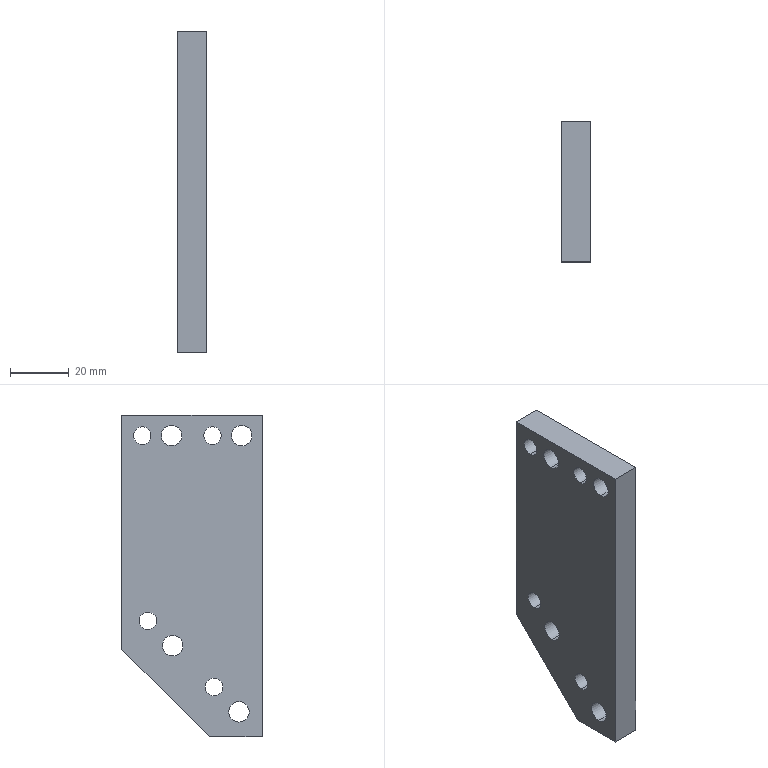Part | STEP file | OP10-140_side plate (F)-R | 1 solid | 23 faces | box 10 x 48 x 110 mm | volume 45630 mm3 | cylinder 16 | plane 7 | commonest cylinder face diameters 6 x8 7 x8